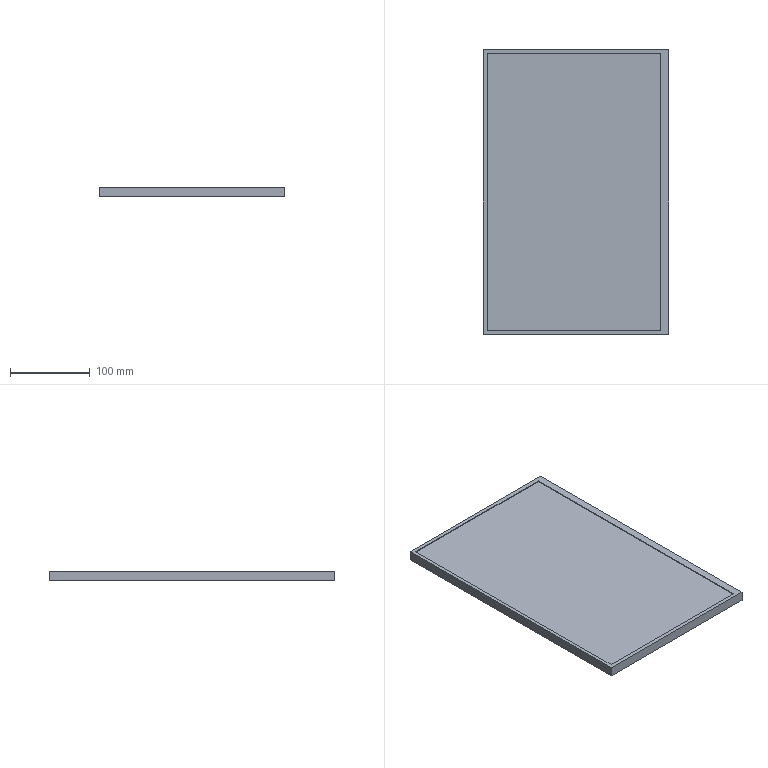Part | STEP file | Operation moving screen V1.201001 | 1 solid | 27 faces | box 232 x 356 x 12.5 mm | volume 957215 mm3 | plane 11 | cylinder 8 | cone 8 | commonest cylinder face diameters 2.5 x8